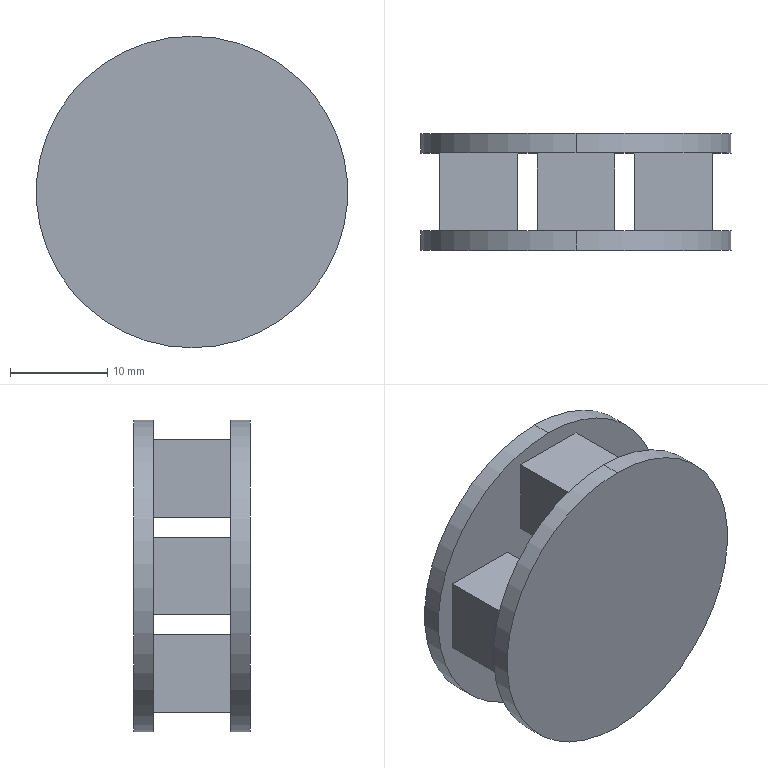Part | SolidWorks | features ICE 2, Extrusion 1 | 1 solid | 24 faces | box 32 x 12 x 32 mm | volume 5265 mm3 | plane 20 | cylinder 4 | commonest cylinder face diameters 32 x4
STEP:
#1=CARTESIAN_POINT('',(0.,12.,-16.));
#2=VERTEX_POINT('',#1);
#3=CARTESIAN_POINT('',(0.,12.,16.));
#4=VERTEX_POINT('',#3);
#5=CARTESIAN_POINT('',(0.,12.,0.));
#6=DIRECTION('',(0.,-1.,0.));
#7=DIRECTION('',(0.,0.,-1.));
#8=AXIS2_PLACEMENT_3D('',#5,#6,#7);
#9=CIRCLE('',#8,16.);
#10=EDGE_CURVE('',#2,#4,#9,.T.);
#11=ORIENTED_EDGE('',*,*,#10,.T.);
#12=CARTESIAN_POINT('',(0.,10.,16.));
#13=VERTEX_POINT('',#12);
#14=CARTESIAN_POINT('',(0.,12.,16.));
#15=DIRECTION('',(0.,-1.,0.));
#16=VECTOR('',#15,1000.);
#17=LINE('',#14,#16);
#18=EDGE_CURVE('',#4,#13,#17,.T.);
#19=ORIENTED_EDGE('',*,*,#18,.T.);
#20=CARTESIAN_POINT('',(0.,10.,-16.));
#21=VERTEX_POINT('',#20);
#22=CARTESIAN_POINT('',(0.,10.,0.));
#23=DIRECTION('',(0.,-1.,0.));
#24=DIRECTION('',(0.,0.,-1.));
#25=AXIS2_PLACEMENT_3D('',#22,#23,#24);
#26=CIRCLE('',#25,16.);
#27=EDGE_CURVE('',#21,#13,#26,.T.);
#28=ORIENTED_EDGE('',*,*,#27,.F.);
#29=CARTESIAN_POINT('',(0.,12.,-16.));
#30=DIRECTION('',(0.,-1.,0.));
#31=VECTOR('',#30,1000.);
#32=LINE('',#29,#31);
#33=EDGE_CURVE('',#2,#21,#32,.T.);
#34=ORIENTED_EDGE('',*,*,#33,.F.);
#35=EDGE_LOOP('',(#11,#19,#28,#34));
#36=FACE_OUTER_BOUND('',#35,.T.);
#37=CARTESIAN_POINT('',(0.,12.,0.));
#38=DIRECTION('',(0.,-1.,0.));
#39=DIRECTION('',(0.,0.,-1.));
#40=AXIS2_PLACEMENT_3D('',#37,#38,#39);
#41=CYLINDRICAL_SURFACE('',#40,16.);
#42=ADVANCED_FACE('',(#36),#41,.T.);
#43=CARTESIAN_POINT('',(0.,2.,16.));
#44=VERTEX_POINT('',#43);
#45=CARTESIAN_POINT('',(0.,2.,-16.));
#46=VERTEX_POINT('',#45);
#47=CARTESIAN_POINT('',(0.,2.,0.));
#48=DIRECTION('',(0.,1.,0.));
#49=DIRECTION('',(0.,0.,1.));
#50=AXIS2_PLACEMENT_3D('',#47,#48,#49);
#51=CIRCLE('',#50,16.);
#52=EDGE_CURVE('',#44,#46,#51,.T.);
#53=ORIENTED_EDGE('',*,*,#52,.F.);
#54=CARTESIAN_POINT('',(0.,0.,16.));
#55=VERTEX_POINT('',#54);
#56=CARTESIAN_POINT('',(0.,2.,16.));
#57=DIRECTION('',(0.,-1.,0.));
#58=VECTOR('',#57,1000.);
#59=LINE('',#56,#58);
#60=EDGE_CURVE('',#44,#55,#59,.T.);
#61=ORIENTED_EDGE('',*,*,#60,.T.);
#62=CARTESIAN_POINT('',(0.,0.,-16.));
#63=VERTEX_POINT('',#62);
#64=CARTESIAN_POINT('',(0.,0.,0.));
#65=DIRECTION('',(0.,1.,0.));
#66=DIRECTION('',(0.,0.,1.));
#67=AXIS2_PLACEMENT_3D('',#64,#65,#66);
#68=CIRCLE('',#67,16.);
#69=EDGE_CURVE('',#55,#63,#68,.T.);
#70=ORIENTED_EDGE('',*,*,#69,.T.);
#71=CARTESIAN_POINT('',(0.,2.,-16.));
#72=DIRECTION('',(0.,-1.,0.));
#73=VECTOR('',#72,1000.);
#74=LINE('',#71,#73);
#75=EDGE_CURVE('',#46,#63,#74,.T.);
#76=ORIENTED_EDGE('',*,*,#75,.F.);
#77=EDGE_LOOP('',(#53,#61,#70,#76));
#78=FACE_OUTER_BOUND('',#77,.T.);
#79=CARTESIAN_POINT('',(0.,2.,0.));
#80=DIRECTION('',(0.,-1.,0.));
#81=DIRECTION('',(0.,0.,-1.));
#82=AXIS2_PLACEMENT_3D('',#79,#80,#81);
#83=CYLINDRICAL_SURFACE('',#82,16.);
#84=ADVANCED_FACE('',(#78),#83,.T.);
#85=CARTESIAN_POINT('',(0.,2.,0.));
#86=DIRECTION('',(0.,1.,0.));
#87=DIRECTION('',(0.,0.,1.));
#88=AXIS2_PLACEMENT_3D('',#85,#86,#87);
#89=CIRCLE('',#88,16.);
#90=EDGE_CURVE('',#46,#44,#89,.T.);
#91=ORIENTED_EDGE('',*,*,#90,.T.);
#92=ORIENTED_EDGE('',*,*,#52,.T.);
#93=EDGE_LOOP('',(#91,#92));
#94=FACE_OUTER_BOUND('',#93,.T.);
#95=CARTESIAN_POINT('',(4.,2.,6.));
#96=VERTEX_POINT('',#95);
#97=CARTESIAN_POINT('',(-4.,2.,6.));
#98=VERTEX_POINT('',#97);
#99=CARTESIAN_POINT('',(-4.,2.,6.));
#100=DIRECTION('',(-1.,0.,0.));
#101=VECTOR('',#100,1000.);
#102=LINE('',#99,#101);
#103=EDGE_CURVE('',#96,#98,#102,.T.);
#104=ORIENTED_EDGE('',*,*,#103,.F.);
#105=CARTESIAN_POINT('',(4.,2.,14.));
#106=VERTEX_POINT('',#105);
#107=CARTESIAN_POINT('',(4.,2.,6.));
#108=DIRECTION('',(0.,0.,-1.));
#109=VECTOR('',#108,1000.);
#110=LINE('',#107,#109);
#111=EDGE_CURVE('',#106,#96,#110,.T.);
#112=ORIENTED_EDGE('',*,*,#111,.F.);
#113=CARTESIAN_POINT('',(-4.,2.,14.));
#114=VERTEX_POINT('',#113);
#115=CARTESIAN_POINT('',(-4.,2.,14.));
#116=DIRECTION('',(1.,0.,0.));
#117=VECTOR('',#116,1000.);
#118=LINE('',#115,#117);
#119=EDGE_CURVE('',#114,#106,#118,.T.);
#120=ORIENTED_EDGE('',*,*,#119,.F.);
#121=CARTESIAN_POINT('',(-4.,2.,6.));
#122=DIRECTION('',(0.,0.,1.));
#123=VECTOR('',#122,1000.);
#124=LINE('',#121,#123);
#125=EDGE_CURVE('',#98,#114,#124,.T.);
#126=ORIENTED_EDGE('',*,*,#125,.F.);
#127=EDGE_LOOP('',(#104,#112,#120,#126));
#128=FACE_BOUND('',#127,.T.);
#129=CARTESIAN_POINT('',(-14.,2.,4.));
#130=VERTEX_POINT('',#129);
#131=CARTESIAN_POINT('',(-6.,2.,4.));
#132=VERTEX_POINT('',#131);
#133=CARTESIAN_POINT('',(-6.,2.,4.));
#134=DIRECTION('',(1.,0.,0.));
#135=VECTOR('',#134,1000.);
#136=LINE('',#133,#135);
#137=EDGE_CURVE('',#130,#132,#136,.T.);
#138=ORIENTED_EDGE('',*,*,#137,.F.);
#139=CARTESIAN_POINT('',(-14.,2.,-4.));
#140=VERTEX_POINT('',#139);
#141=CARTESIAN_POINT('',(-14.,2.,-4.));
#142=DIRECTION('',(0.,0.,1.));
#143=VECTOR('',#142,1000.);
#144=LINE('',#141,#143);
#145=EDGE_CURVE('',#140,#130,#144,.T.);
#146=ORIENTED_EDGE('',*,*,#145,.F.);
#147=CARTESIAN_POINT('',(-6.,2.,-4.));
#148=VERTEX_POINT('',#147);
#149=CARTESIAN_POINT('',(-6.,2.,-4.));
#150=DIRECTION('',(-1.,0.,0.));
#151=VECTOR('',#150,1000.);
#152=LINE('',#149,#151);
#153=EDGE_CURVE('',#148,#140,#152,.T.);
#154=ORIENTED_EDGE('',*,*,#153,.F.);
#155=CARTESIAN_POINT('',(-6.,2.,-4.));
#156=DIRECTION('',(0.,0.,-1.));
#157=VECTOR('',#156,1000.);
#158=LINE('',#155,#157);
#159=EDGE_CURVE('',#132,#148,#158,.T.);
#160=ORIENTED_EDGE('',*,*,#159,.F.);
#161=EDGE_LOOP('',(#138,#146,#154,#160));
#162=FACE_BOUND('',#161,.T.);
#163=CARTESIAN_POINT('',(-4.,2.,-14.));
#164=VERTEX_POINT('',#163);
#165=CARTESIAN_POINT('',(-4.,2.,-6.));
#166=VERTEX_POINT('',#165);
#167=CARTESIAN_POINT('',(-4.,2.,-6.));
#168=DIRECTION('',(0.,0.,1.));
#169=VECTOR('',#168,1000.);
#170=LINE('',#167,#169);
#171=EDGE_CURVE('',#164,#166,#170,.T.);
#172=ORIENTED_EDGE('',*,*,#171,.F.);
#173=CARTESIAN_POINT('',(4.,2.,-14.));
#174=VERTEX_POINT('',#173);
#175=CARTESIAN_POINT('',(4.,2.,-14.));
#176=DIRECTION('',(-1.,0.,0.));
#177=VECTOR('',#176,1000.);
#178=LINE('',#175,#177);
#179=EDGE_CURVE('',#174,#164,#178,.T.);
#180=ORIENTED_EDGE('',*,*,#179,.F.);
#181=CARTESIAN_POINT('',(4.,2.,-6.));
#182=VERTEX_POINT('',#181);
#183=CARTESIAN_POINT('',(4.,2.,-6.));
#184=DIRECTION('',(0.,0.,-1.));
#185=VECTOR('',#184,1000.);
#186=LINE('',#183,#185);
#187=EDGE_CURVE('',#182,#174,#186,.T.);
#188=ORIENTED_EDGE('',*,*,#187,.F.);
#189=CARTESIAN_POINT('',(4.,2.,-6.));
#190=DIRECTION('',(1.,0.,0.));
#191=VECTOR('',#190,1000.);
#192=LINE('',#189,#191);
#193=EDGE_CURVE('',#166,#182,#192,.T.);
#194=ORIENTED_EDGE('',*,*,#193,.F.);
#195=EDGE_LOOP('',(#172,#180,#188,#194));
#196=FACE_BOUND('',#195,.T.);
#197=CARTESIAN_POINT('',(14.,2.,-4.));
#198=VERTEX_POINT('',#197);
#199=CARTESIAN_POINT('',(6.,2.,-4.));
#200=VERTEX_POINT('',#199);
#201=CARTESIAN_POINT('',(6.,2.,-4.));
#202=DIRECTION('',(-1.,0.,0.));
#203=VECTOR('',#202,1000.);
#204=LINE('',#201,#203);
#205=EDGE_CURVE('',#198,#200,#204,.T.);
#206=ORIENTED_EDGE('',*,*,#205,.F.);
#207=CARTESIAN_POINT('',(14.,2.,4.));
#208=VERTEX_POINT('',#207);
#209=CARTESIAN_POINT('',(14.,2.,4.));
#210=DIRECTION('',(0.,0.,-1.));
#211=VECTOR('',#210,1000.);
#212=LINE('',#209,#211);
#213=EDGE_CURVE('',#208,#198,#212,.T.);
#214=ORIENTED_EDGE('',*,*,#213,.F.);
#215=CARTESIAN_POINT('',(6.,2.,4.));
#216=VERTEX_POINT('',#215);
#217=CARTESIAN_POINT('',(6.,2.,4.));
#218=DIRECTION('',(1.,0.,0.));
#219=VECTOR('',#218,1000.);
#220=LINE('',#217,#219);
#221=EDGE_CURVE('',#216,#208,#220,.T.);
#222=ORIENTED_EDGE('',*,*,#221,.F.);
#223=CARTESIAN_POINT('',(6.,2.,4.));
#224=DIRECTION('',(0.,0.,1.));
#225=VECTOR('',#224,1000.);
#226=LINE('',#223,#225);
#227=EDGE_CURVE('',#200,#216,#226,.T.);
#228=ORIENTED_EDGE('',*,*,#227,.F.);
#229=EDGE_LOOP('',(#206,#214,#222,#228));
#230=FACE_BOUND('',#229,.T.);
#231=CARTESIAN_POINT('',(0.,2.,0.));
#232=DIRECTION('',(0.,1.,0.));
#233=DIRECTION('',(0.,0.,1.));
#234=AXIS2_PLACEMENT_3D('',#231,#232,#233);
#235=PLANE('',#234);
#236=ADVANCED_FACE('',(#94,#128,#162,#196,#230),#235,.T.);
#237=ORIENTED_EDGE('',*,*,#60,.F.);
#238=ORIENTED_EDGE('',*,*,#90,.F.);
#239=ORIENTED_EDGE('',*,*,#75,.T.);
#240=CARTESIAN_POINT('',(0.,0.,0.));
#241=DIRECTION('',(0.,1.,0.));
#242=DIRECTION('',(0.,0.,1.));
#243=AXIS2_PLACEMENT_3D('',#240,#241,#242);
#244=CIRCLE('',#243,16.);
#245=EDGE_CURVE('',#63,#55,#244,.T.);
#246=ORIENTED_EDGE('',*,*,#245,.T.);
#247=EDGE_LOOP('',(#237,#238,#239,#246));
#248=FACE_OUTER_BOUND('',#247,.T.);
#249=CARTESIAN_POINT('',(0.,2.,0.));
#250=DIRECTION('',(0.,-1.,0.));
#251=DIRECTION('',(0.,0.,-1.));
#252=AXIS2_PLACEMENT_3D('',#249,#250,#251);
#253=CYLINDRICAL_SURFACE('',#252,16.);
#254=ADVANCED_FACE('',(#248),#253,.T.);
#255=ORIENTED_EDGE('',*,*,#245,.F.);
#256=ORIENTED_EDGE('',*,*,#69,.F.);
#257=EDGE_LOOP('',(#255,#256));
#258=FACE_OUTER_BOUND('',#257,.T.);
#259=CARTESIAN_POINT('',(0.,0.,0.));
#260=DIRECTION('',(0.,1.,0.));
#261=DIRECTION('',(0.,0.,1.));
#262=AXIS2_PLACEMENT_3D('',#259,#260,#261);
#263=PLANE('',#262);
#264=ADVANCED_FACE('',(#258),#263,.F.);
#265=ORIENTED_EDGE('',*,*,#111,.T.);
#266=CARTESIAN_POINT('',(4.,10.,6.));
#267=VERTEX_POINT('',#266);
#268=CARTESIAN_POINT('',(4.,10.,6.));
#269=DIRECTION('',(0.,-1.,0.));
#270=VECTOR('',#269,1000.);
#271=LINE('',#268,#270);
#272=EDGE_CURVE('',#267,#96,#271,.T.);
#273=ORIENTED_EDGE('',*,*,#272,.F.);
#274=CARTESIAN_POINT('',(4.,10.,14.));
#275=VERTEX_POINT('',#274);
#276=CARTESIAN_POINT('',(4.,10.,6.));
#277=DIRECTION('',(0.,0.,-1.));
#278=VECTOR('',#277,1000.);
#279=LINE('',#276,#278);
#280=EDGE_CURVE('',#275,#267,#279,.T.);
#281=ORIENTED_EDGE('',*,*,#280,.F.);
#282=CARTESIAN_POINT('',(4.,10.,14.));
#283=DIRECTION('',(0.,-1.,0.));
#284=VECTOR('',#283,1000.);
#285=LINE('',#282,#284);
#286=EDGE_CURVE('',#275,#106,#285,.T.);
#287=ORIENTED_EDGE('',*,*,#286,.T.);
#288=EDGE_LOOP('',(#265,#273,#281,#287));
#289=FACE_OUTER_BOUND('',#288,.T.);
#290=CARTESIAN_POINT('',(4.,10.,6.));
#291=DIRECTION('',(-1.,0.,0.));
#292=DIRECTION('',(0.,0.,1.));
#293=AXIS2_PLACEMENT_3D('',#290,#291,#292);
#294=PLANE('',#293);
#295=ADVANCED_FACE('',(#289),#294,.F.);
#296=ORIENTED_EDGE('',*,*,#103,.T.);
#297=CARTESIAN_POINT('',(-4.,10.,6.));
#298=VERTEX_POINT('',#297);
#299=CARTESIAN_POINT('',(-4.,10.,6.));
#300=DIRECTION('',(0.,-1.,0.));
#301=VECTOR('',#300,1000.);
#302=LINE('',#299,#301);
#303=EDGE_CURVE('',#298,#98,#302,.T.);
#304=ORIENTED_EDGE('',*,*,#303,.F.);
#305=CARTESIAN_POINT('',(-4.,10.,6.));
#306=DIRECTION('',(-1.,0.,0.));
#307=VECTOR('',#306,1000.);
#308=LINE('',#305,#307);
#309=EDGE_CURVE('',#267,#298,#308,.T.);
#310=ORIENTED_EDGE('',*,*,#309,.F.);
#311=ORIENTED_EDGE('',*,*,#272,.T.);
#312=EDGE_LOOP('',(#296,#304,#310,#311));
#313=FACE_OUTER_BOUND('',#312,.T.);
#314=CARTESIAN_POINT('',(-4.,10.,6.));
#315=DIRECTION('',(0.,0.,1.));
#316=DIRECTION('',(1.,0.,0.));
#317=AXIS2_PLACEMENT_3D('',#314,#315,#316);
#318=PLANE('',#317);
#319=ADVANCED_FACE('',(#313),#318,.F.);
#320=ORIENTED_EDGE('',*,*,#125,.T.);
#321=CARTESIAN_POINT('',(-4.,10.,14.));
#322=VERTEX_POINT('',#321);
#323=CARTESIAN_POINT('',(-4.,10.,14.));
#324=DIRECTION('',(0.,-1.,0.));
#325=VECTOR('',#324,1000.);
#326=LINE('',#323,#325);
#327=EDGE_CURVE('',#322,#114,#326,.T.);
#328=ORIENTED_EDGE('',*,*,#327,.F.);
#329=CARTESIAN_POINT('',(-4.,10.,6.));
#330=DIRECTION('',(0.,0.,1.));
#331=VECTOR('',#330,1000.);
#332=LINE('',#329,#331);
#333=EDGE_CURVE('',#298,#322,#332,.T.);
#334=ORIENTED_EDGE('',*,*,#333,.F.);
#335=ORIENTED_EDGE('',*,*,#303,.T.);
#336=EDGE_LOOP('',(#320,#328,#334,#335));
#337=FACE_OUTER_BOUND('',#336,.T.);
#338=CARTESIAN_POINT('',(-4.,10.,6.));
#339=DIRECTION('',(1.,0.,0.));
#340=DIRECTION('',(0.,0.,-1.));
#341=AXIS2_PLACEMENT_3D('',#338,#339,#340);
#342=PLANE('',#341);
#343=ADVANCED_FACE('',(#337),#342,.F.);
#344=ORIENTED_EDGE('',*,*,#119,.T.);
#345=ORIENTED_EDGE('',*,*,#286,.F.);
#346=CARTESIAN_POINT('',(-4.,10.,14.));
#347=DIRECTION('',(1.,0.,0.));
#348=VECTOR('',#347,1000.);
#349=LINE('',#346,#348);
#350=EDGE_CURVE('',#322,#275,#349,.T.);
#351=ORIENTED_EDGE('',*,*,#350,.F.);
#352=ORIENTED_EDGE('',*,*,#327,.T.);
#353=EDGE_LOOP('',(#344,#345,#351,#352));
#354=FACE_OUTER_BOUND('',#353,.T.);
#355=CARTESIAN_POINT('',(-4.,10.,14.));
#356=DIRECTION('',(0.,0.,-1.));
#357=DIRECTION('',(-1.,0.,0.));
#358=AXIS2_PLACEMENT_3D('',#355,#356,#357);
#359=PLANE('',#358);
#360=ADVANCED_FACE('',(#354),#359,.F.);
#361=ORIENTED_EDGE('',*,*,#145,.T.);
#362=CARTESIAN_POINT('',(-14.,10.,4.));
#363=VERTEX_POINT('',#362);
#364=CARTESIAN_POINT('',(-14.,10.,4.));
#365=DIRECTION('',(0.,-1.,0.));
#366=VECTOR('',#365,1000.);
#367=LINE('',#364,#366);
#368=EDGE_CURVE('',#363,#130,#367,.T.);
#369=ORIENTED_EDGE('',*,*,#368,.F.);
#370=CARTESIAN_POINT('',(-14.,10.,-4.));
#371=VERTEX_POINT('',#370);
#372=CARTESIAN_POINT('',(-14.,10.,-4.));
#373=DIRECTION('',(0.,0.,1.));
#374=VECTOR('',#373,1000.);
#375=LINE('',#372,#374);
#376=EDGE_CURVE('',#371,#363,#375,.T.);
#377=ORIENTED_EDGE('',*,*,#376,.F.);
#378=CARTESIAN_POINT('',(-14.,10.,-4.));
#379=DIRECTION('',(0.,-1.,0.));
#380=VECTOR('',#379,1000.);
#381=LINE('',#378,#380);
#382=EDGE_CURVE('',#371,#140,#381,.T.);
#383=ORIENTED_EDGE('',*,*,#382,.T.);
#384=EDGE_LOOP('',(#361,#369,#377,#383));
#385=FACE_OUTER_BOUND('',#384,.T.);
#386=CARTESIAN_POINT('',(-14.,10.,-4.));
#387=DIRECTION('',(1.,0.,0.));
#388=DIRECTION('',(0.,0.,-1.));
#389=AXIS2_PLACEMENT_3D('',#386,#387,#388);
#390=PLANE('',#389);
#391=ADVANCED_FACE('',(#385),#390,.F.);
#392=ORIENTED_EDGE('',*,*,#137,.T.);
#393=CARTESIAN_POINT('',(-6.,10.,4.));
#394=VERTEX_POINT('',#393);
#395=CARTESIAN_POINT('',(-6.,10.,4.));
#396=DIRECTION('',(0.,-1.,0.));
#397=VECTOR('',#396,1000.);
#398=LINE('',#395,#397);
#399=EDGE_CURVE('',#394,#132,#398,.T.);
#400=ORIENTED_EDGE('',*,*,#399,.F.);
#401=CARTESIAN_POINT('',(-6.,10.,4.));
#402=DIRECTION('',(1.,0.,0.));
#403=VECTOR('',#402,1000.);
#404=LINE('',#401,#403);
#405=EDGE_CURVE('',#363,#394,#404,.T.);
#406=ORIENTED_EDGE('',*,*,#405,.F.);
#407=ORIENTED_EDGE('',*,*,#368,.T.);
#408=EDGE_LOOP('',(#392,#400,#406,#407));
#409=FACE_OUTER_BOUND('',#408,.T.);
#410=CARTESIAN_POINT('',(-6.,10.,4.));
#411=DIRECTION('',(0.,0.,-1.));
#412=DIRECTION('',(-1.,0.,0.));
#413=AXIS2_PLACEMENT_3D('',#410,#411,#412);
#414=PLANE('',#413);
#415=ADVANCED_FACE('',(#409),#414,.F.);
#416=ORIENTED_EDGE('',*,*,#159,.T.);
#417=CARTESIAN_POINT('',(-6.,10.,-4.));
#418=VERTEX_POINT('',#417);
#419=CARTESIAN_POINT('',(-6.,10.,-4.));
#420=DIRECTION('',(0.,-1.,0.));
#421=VECTOR('',#420,1000.);
#422=LINE('',#419,#421);
#423=EDGE_CURVE('',#418,#148,#422,.T.);
#424=ORIENTED_EDGE('',*,*,#423,.F.);
#425=CARTESIAN_POINT('',(-6.,10.,-4.));
#426=DIRECTION('',(0.,0.,-1.));
#427=VECTOR('',#426,1000.);
#428=LINE('',#425,#427);
#429=EDGE_CURVE('',#394,#418,#428,.T.);
#430=ORIENTED_EDGE('',*,*,#429,.F.);
#431=ORIENTED_EDGE('',*,*,#399,.T.);
#432=EDGE_LOOP('',(#416,#424,#430,#431));
#433=FACE_OUTER_BOUND('',#432,.T.);
#434=CARTESIAN_POINT('',(-6.,10.,-4.));
#435=DIRECTION('',(-1.,0.,0.));
#436=DIRECTION('',(0.,0.,1.));
#437=AXIS2_PLACEMENT_3D('',#434,#435,#436);
#438=PLANE('',#437);
#439=ADVANCED_FACE('',(#433),#438,.F.);
#440=ORIENTED_EDGE('',*,*,#153,.T.);
#441=ORIENTED_EDGE('',*,*,#382,.F.);
#442=CARTESIAN_POINT('',(-6.,10.,-4.));
#443=DIRECTION('',(-1.,0.,0.));
#444=VECTOR('',#443,1000.);
#445=LINE('',#442,#444);
#446=EDGE_CURVE('',#418,#371,#445,.T.);
#447=ORIENTED_EDGE('',*,*,#446,.F.);
#448=ORIENTED_EDGE('',*,*,#423,.T.);
#449=EDGE_LOOP('',(#440,#441,#447,#448));
#450=FACE_OUTER_BOUND('',#449,.T.);
#451=CARTESIAN_POINT('',(-6.,10.,-4.));
#452=DIRECTION('',(0.,0.,1.));
#453=DIRECTION('',(1.,0.,0.));
#454=AXIS2_PLACEMENT_3D('',#451,#452,#453);
#455=PLANE('',#454);
#456=ADVANCED_FACE('',(#450),#455,.F.);
#457=ORIENTED_EDGE('',*,*,#179,.T.);
#458=CARTESIAN_POINT('',(-4.,10.,-14.));
#459=VERTEX_POINT('',#458);
#460=CARTESIAN_POINT('',(-4.,10.,-14.));
#461=DIRECTION('',(0.,-1.,0.));
#462=VECTOR('',#461,1000.);
#463=LINE('',#460,#462);
#464=EDGE_CURVE('',#459,#164,#463,.T.);
#465=ORIENTED_EDGE('',*,*,#464,.F.);
#466=CARTESIAN_POINT('',(4.,10.,-14.));
#467=VERTEX_POINT('',#466);
#468=CARTESIAN_POINT('',(4.,10.,-14.));
#469=DIRECTION('',(-1.,0.,0.));
#470=VECTOR('',#469,1000.);
#471=LINE('',#468,#470);
#472=EDGE_CURVE('',#467,#459,#471,.T.);
#473=ORIENTED_EDGE('',*,*,#472,.F.);
#474=CARTESIAN_POINT('',(4.,10.,-14.));
#475=DIRECTION('',(0.,-1.,0.));
#476=VECTOR('',#475,1000.);
#477=LINE('',#474,#476);
#478=EDGE_CURVE('',#467,#174,#477,.T.);
#479=ORIENTED_EDGE('',*,*,#478,.T.);
#480=EDGE_LOOP('',(#457,#465,#473,#479));
#481=FACE_OUTER_BOUND('',#480,.T.);
#482=CARTESIAN_POINT('',(4.,10.,-14.));
#483=DIRECTION('',(0.,0.,1.));
#484=DIRECTION('',(1.,0.,0.));
#485=AXIS2_PLACEMENT_3D('',#482,#483,#484);
#486=PLANE('',#485);
#487=ADVANCED_FACE('',(#481),#486,.F.);
#488=ORIENTED_EDGE('',*,*,#171,.T.);
#489=CARTESIAN_POINT('',(-4.,10.,-6.));
#490=VERTEX_POINT('',#489);
#491=CARTESIAN_POINT('',(-4.,10.,-6.));
#492=DIRECTION('',(0.,-1.,0.));
#493=VECTOR('',#492,1000.);
#494=LINE('',#491,#493);
#495=EDGE_CURVE('',#490,#166,#494,.T.);
#496=ORIENTED_EDGE('',*,*,#495,.F.);
#497=CARTESIAN_POINT('',(-4.,10.,-6.));
#498=DIRECTION('',(0.,0.,1.));
#499=VECTOR('',#498,1000.);
#500=LINE('',#497,#499);
#501=EDGE_CURVE('',#459,#490,#500,.T.);
#502=ORIENTED_EDGE('',*,*,#501,.F.);
#503=ORIENTED_EDGE('',*,*,#464,.T.);
#504=EDGE_LOOP('',(#488,#496,#502,#503));
#505=FACE_OUTER_BOUND('',#504,.T.);
#506=CARTESIAN_POINT('',(-4.,10.,-6.));
#507=DIRECTION('',(1.,0.,0.));
#508=DIRECTION('',(0.,0.,-1.));
#509=AXIS2_PLACEMENT_3D('',#506,#507,#508);
#510=PLANE('',#509);
#511=ADVANCED_FACE('',(#505),#510,.F.);
#512=ORIENTED_EDGE('',*,*,#193,.T.);
#513=CARTESIAN_POINT('',(4.,10.,-6.));
#514=VERTEX_POINT('',#513);
#515=CARTESIAN_POINT('',(4.,10.,-6.));
#516=DIRECTION('',(0.,-1.,0.));
#517=VECTOR('',#516,1000.);
#518=LINE('',#515,#517);
#519=EDGE_CURVE('',#514,#182,#518,.T.);
#520=ORIENTED_EDGE('',*,*,#519,.F.);
#521=CARTESIAN_POINT('',(4.,10.,-6.));
#522=DIRECTION('',(1.,0.,0.));
#523=VECTOR('',#522,1000.);
#524=LINE('',#521,#523);
#525=EDGE_CURVE('',#490,#514,#524,.T.);
#526=ORIENTED_EDGE('',*,*,#525,.F.);
#527=ORIENTED_EDGE('',*,*,#495,.T.);
#528=EDGE_LOOP('',(#512,#520,#526,#527));
#529=FACE_OUTER_BOUND('',#528,.T.);
#530=CARTESIAN_POINT('',(4.,10.,-6.));
#531=DIRECTION('',(0.,0.,-1.));
#532=DIRECTION('',(-1.,0.,0.));
#533=AXIS2_PLACEMENT_3D('',#530,#531,#532);
#534=PLANE('',#533);
#535=ADVANCED_FACE('',(#529),#534,.F.);
#536=ORIENTED_EDGE('',*,*,#187,.T.);
#537=ORIENTED_EDGE('',*,*,#478,.F.);
#538=CARTESIAN_POINT('',(4.,10.,-6.));
#539=DIRECTION('',(0.,0.,-1.));
#540=VECTOR('',#539,1000.);
#541=LINE('',#538,#540);
#542=EDGE_CURVE('',#514,#467,#541,.T.);
#543=ORIENTED_EDGE('',*,*,#542,.F.);
#544=ORIENTED_EDGE('',*,*,#519,.T.);
#545=EDGE_LOOP('',(#536,#537,#543,#544));
#546=FACE_OUTER_BOUND('',#545,.T.);
#547=CARTESIAN_POINT('',(4.,10.,-6.));
#548=DIRECTION('',(-1.,0.,0.));
#549=DIRECTION('',(0.,0.,1.));
#550=AXIS2_PLACEMENT_3D('',#547,#548,#549);
#551=PLANE('',#550);
#552=ADVANCED_FACE('',(#546),#551,.F.);
#553=ORIENTED_EDGE('',*,*,#213,.T.);
#554=CARTESIAN_POINT('',(14.,10.,-4.));
#555=VERTEX_POINT('',#554);
#556=CARTESIAN_POINT('',(14.,10.,-4.));
#557=DIRECTION('',(0.,-1.,0.));
#558=VECTOR('',#557,1000.);
#559=LINE('',#556,#558);
#560=EDGE_CURVE('',#555,#198,#559,.T.);
#561=ORIENTED_EDGE('',*,*,#560,.F.);
#562=CARTESIAN_POINT('',(14.,10.,4.));
#563=VERTEX_POINT('',#562);
#564=CARTESIAN_POINT('',(14.,10.,4.));
#565=DIRECTION('',(0.,0.,-1.));
#566=VECTOR('',#565,1000.);
#567=LINE('',#564,#566);
#568=EDGE_CURVE('',#563,#555,#567,.T.);
#569=ORIENTED_EDGE('',*,*,#568,.F.);
#570=CARTESIAN_POINT('',(14.,10.,4.));
#571=DIRECTION('',(0.,-1.,0.));
#572=VECTOR('',#571,1000.);
#573=LINE('',#570,#572);
#574=EDGE_CURVE('',#563,#208,#573,.T.);
#575=ORIENTED_EDGE('',*,*,#574,.T.);
#576=EDGE_LOOP('',(#553,#561,#569,#575));
#577=FACE_OUTER_BOUND('',#576,.T.);
#578=CARTESIAN_POINT('',(14.,10.,4.));
#579=DIRECTION('',(-1.,0.,0.));
#580=DIRECTION('',(0.,0.,1.));
#581=AXIS2_PLACEMENT_3D('',#578,#579,#580);
#582=PLANE('',#581);
#583=ADVANCED_FACE('',(#577),#582,.F.);
#584=ORIENTED_EDGE('',*,*,#205,.T.);
#585=CARTESIAN_POINT('',(6.,10.,-4.));
#586=VERTEX_POINT('',#585);
#587=CARTESIAN_POINT('',(6.,10.,-4.));
#588=DIRECTION('',(0.,-1.,0.));
#589=VECTOR('',#588,1000.);
#590=LINE('',#587,#589);
#591=EDGE_CURVE('',#586,#200,#590,.T.);
#592=ORIENTED_EDGE('',*,*,#591,.F.);
#593=CARTESIAN_POINT('',(6.,10.,-4.));
#594=DIRECTION('',(-1.,0.,0.));
#595=VECTOR('',#594,1000.);
#596=LINE('',#593,#595);
#597=EDGE_CURVE('',#555,#586,#596,.T.);
#598=ORIENTED_EDGE('',*,*,#597,.F.);
#599=ORIENTED_EDGE('',*,*,#560,.T.);
#600=EDGE_LOOP('',(#584,#592,#598,#599));
#601=FACE_OUTER_BOUND('',#600,.T.);
#602=CARTESIAN_POINT('',(6.,10.,-4.));
#603=DIRECTION('',(0.,0.,1.));
#604=DIRECTION('',(1.,0.,0.));
#605=AXIS2_PLACEMENT_3D('',#602,#603,#604);
#606=PLANE('',#605);
#607=ADVANCED_FACE('',(#601),#606,.F.);
#608=ORIENTED_EDGE('',*,*,#227,.T.);
#609=CARTESIAN_POINT('',(6.,10.,4.));
#610=VERTEX_POINT('',#609);
#611=CARTESIAN_POINT('',(6.,10.,4.));
#612=DIRECTION('',(0.,-1.,0.));
#613=VECTOR('',#612,1000.);
#614=LINE('',#611,#613);
#615=EDGE_CURVE('',#610,#216,#614,.T.);
#616=ORIENTED_EDGE('',*,*,#615,.F.);
#617=CARTESIAN_POINT('',(6.,10.,4.));
#618=DIRECTION('',(0.,0.,1.));
#619=VECTOR('',#618,1000.);
#620=LINE('',#617,#619);
#621=EDGE_CURVE('',#586,#610,#620,.T.);
#622=ORIENTED_EDGE('',*,*,#621,.F.);
#623=ORIENTED_EDGE('',*,*,#591,.T.);
#624=EDGE_LOOP('',(#608,#616,#622,#623));
#625=FACE_OUTER_BOUND('',#624,.T.);
#626=CARTESIAN_POINT('',(6.,10.,4.));
#627=DIRECTION('',(1.,0.,0.));
#628=DIRECTION('',(0.,0.,-1.));
#629=AXIS2_PLACEMENT_3D('',#626,#627,#628);
#630=PLANE('',#629);
#631=ADVANCED_FACE('',(#625),#630,.F.);
#632=ORIENTED_EDGE('',*,*,#221,.T.);
#633=ORIENTED_EDGE('',*,*,#574,.F.);
#634=CARTESIAN_POINT('',(6.,10.,4.));
#635=DIRECTION('',(1.,0.,0.));
#636=VECTOR('',#635,1000.);
#637=LINE('',#634,#636);
#638=EDGE_CURVE('',#610,#563,#637,.T.);
#639=ORIENTED_EDGE('',*,*,#638,.F.);
#640=ORIENTED_EDGE('',*,*,#615,.T.);
#641=EDGE_LOOP('',(#632,#633,#639,#640));
#642=FACE_OUTER_BOUND('',#641,.T.);
#643=CARTESIAN_POINT('',(6.,10.,4.));
#644=DIRECTION('',(0.,0.,-1.));
#645=DIRECTION('',(-1.,0.,0.));
#646=AXIS2_PLACEMENT_3D('',#643,#644,#645);
#647=PLANE('',#646);
#648=ADVANCED_FACE('',(#642),#647,.F.);
#649=ORIENTED_EDGE('',*,*,#18,.F.);
#650=CARTESIAN_POINT('',(0.,12.,0.));
#651=DIRECTION('',(0.,-1.,0.));
#652=DIRECTION('',(0.,0.,-1.));
#653=AXIS2_PLACEMENT_3D('',#650,#651,#652);
#654=CIRCLE('',#653,16.);
#655=EDGE_CURVE('',#4,#2,#654,.T.);
#656=ORIENTED_EDGE('',*,*,#655,.T.);
#657=ORIENTED_EDGE('',*,*,#33,.T.);
#658=CARTESIAN_POINT('',(0.,10.,0.));
#659=DIRECTION('',(0.,-1.,0.));
#660=DIRECTION('',(0.,0.,-1.));
#661=AXIS2_PLACEMENT_3D('',#658,#659,#660);
#662=CIRCLE('',#661,16.);
#663=EDGE_CURVE('',#13,#21,#662,.T.);
#664=ORIENTED_EDGE('',*,*,#663,.F.);
#665=EDGE_LOOP('',(#649,#656,#657,#664));
#666=FACE_OUTER_BOUND('',#665,.T.);
#667=CARTESIAN_POINT('',(0.,12.,0.));
#668=DIRECTION('',(0.,-1.,0.));
#669=DIRECTION('',(0.,0.,-1.));
#670=AXIS2_PLACEMENT_3D('',#667,#668,#669);
#671=CYLINDRICAL_SURFACE('',#670,16.);
#672=ADVANCED_FACE('',(#666),#671,.T.);
#673=ORIENTED_EDGE('',*,*,#10,.F.);
#674=ORIENTED_EDGE('',*,*,#655,.F.);
#675=EDGE_LOOP('',(#673,#674));
#676=FACE_OUTER_BOUND('',#675,.T.);
#677=CARTESIAN_POINT('',(0.,12.,0.));
#678=DIRECTION('',(0.,-1.,0.));
#679=DIRECTION('',(0.,0.,-1.));
#680=AXIS2_PLACEMENT_3D('',#677,#678,#679);
#681=PLANE('',#680);
#682=ADVANCED_FACE('',(#676),#681,.F.);
#683=ORIENTED_EDGE('',*,*,#350,.T.);
#684=ORIENTED_EDGE('',*,*,#280,.T.);
#685=ORIENTED_EDGE('',*,*,#309,.T.);
#686=ORIENTED_EDGE('',*,*,#333,.T.);
#687=EDGE_LOOP('',(#683,#684,#685,#686));
#688=FACE_BOUND('',#687,.T.);
#689=ORIENTED_EDGE('',*,*,#446,.T.);
#690=ORIENTED_EDGE('',*,*,#376,.T.);
#691=ORIENTED_EDGE('',*,*,#405,.T.);
#692=ORIENTED_EDGE('',*,*,#429,.T.);
#693=EDGE_LOOP('',(#689,#690,#691,#692));
#694=FACE_BOUND('',#693,.T.);
#695=ORIENTED_EDGE('',*,*,#542,.T.);
#696=ORIENTED_EDGE('',*,*,#472,.T.);
#697=ORIENTED_EDGE('',*,*,#501,.T.);
#698=ORIENTED_EDGE('',*,*,#525,.T.);
#699=EDGE_LOOP('',(#695,#696,#697,#698));
#700=FACE_BOUND('',#699,.T.);
#701=ORIENTED_EDGE('',*,*,#638,.T.);
#702=ORIENTED_EDGE('',*,*,#568,.T.);
#703=ORIENTED_EDGE('',*,*,#597,.T.);
#704=ORIENTED_EDGE('',*,*,#621,.T.);
#705=EDGE_LOOP('',(#701,#702,#703,#704));
#706=FACE_BOUND('',#705,.T.);
#707=ORIENTED_EDGE('',*,*,#27,.T.);
#708=ORIENTED_EDGE('',*,*,#663,.T.);
#709=EDGE_LOOP('',(#707,#708));
#710=FACE_OUTER_BOUND('',#709,.T.);
#711=CARTESIAN_POINT('',(0.,10.,0.));
#712=DIRECTION('',(0.,-1.,0.));
#713=DIRECTION('',(0.,0.,-1.));
#714=AXIS2_PLACEMENT_3D('',#711,#712,#713);
#715=PLANE('',#714);
#716=ADVANCED_FACE('',(#688,#694,#700,#706,#710),#715,.T.);
#717=CLOSED_SHELL('',(#42,#84,#236,#254,#264,#295,#319,#343,#360,#391,#415,#439,#456,#487,#511,#535,#552,#583,#607,#631,#648,#672,#682,#716));
#718=MANIFOLD_SOLID_BREP('',#717);
#719=CARTESIAN_POINT('',(0.,0.,0.));
#720=DIRECTION('',(0.,0.,1.));
#721=DIRECTION('',(1.,0.,0.));
#722=AXIS2_PLACEMENT_3D('',#719,#720,#721);
#723=(LENGTH_UNIT()NAMED_UNIT(*)SI_UNIT(.MILLI.,.METRE.));
#724=UNCERTAINTY_MEASURE_WITH_UNIT(LENGTH_MEASURE(0.00001),#723,'','');
#725=(NAMED_UNIT(*)PLANE_ANGLE_UNIT()SI_UNIT($,.RADIAN.));
#726=(NAMED_UNIT(*)SI_UNIT($,.STERADIAN.)SOLID_ANGLE_UNIT());
#727=(GEOMETRIC_REPRESENTATION_CONTEXT(3)GLOBAL_UNCERTAINTY_ASSIGNED_CONTEXT((#724))GLOBAL_UNIT_ASSIGNED_CONTEXT((#723,#725,#726))REPRESENTATION_CONTEXT('',''));
#728=ADVANCED_BREP_SHAPE_REPRESENTATION('',(#718,#722),#727);